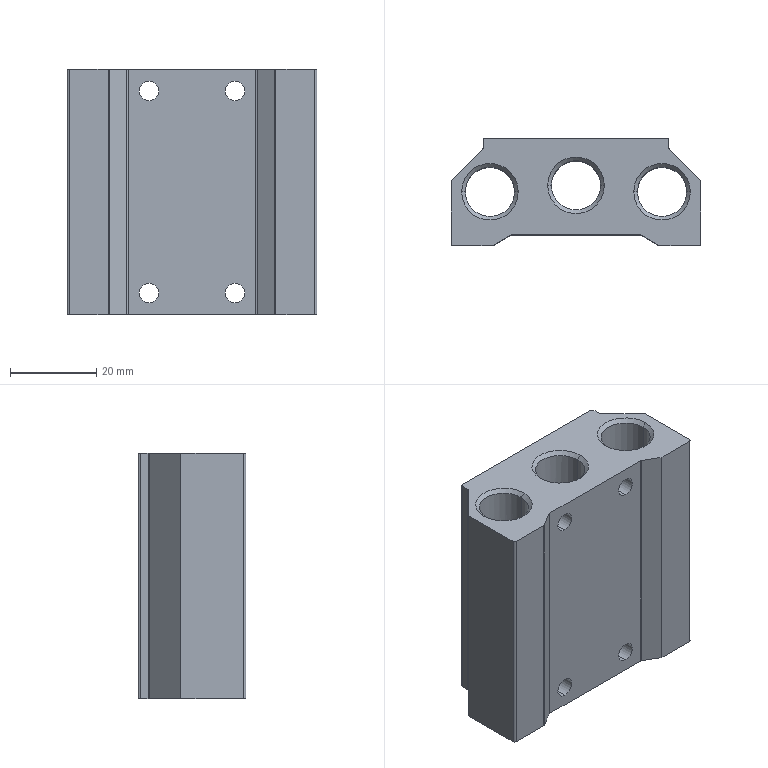Part | STEP file | 100M-2F | 1 solid | 90 faces | box 58 x 25 x 57 mm | volume 50604 mm3 | cylinder 44 | cone 28 | plane 18 | commonest cylinder face diameters 8 x12 1 x10 2.459 x8 4.5 x8 11.445 x6